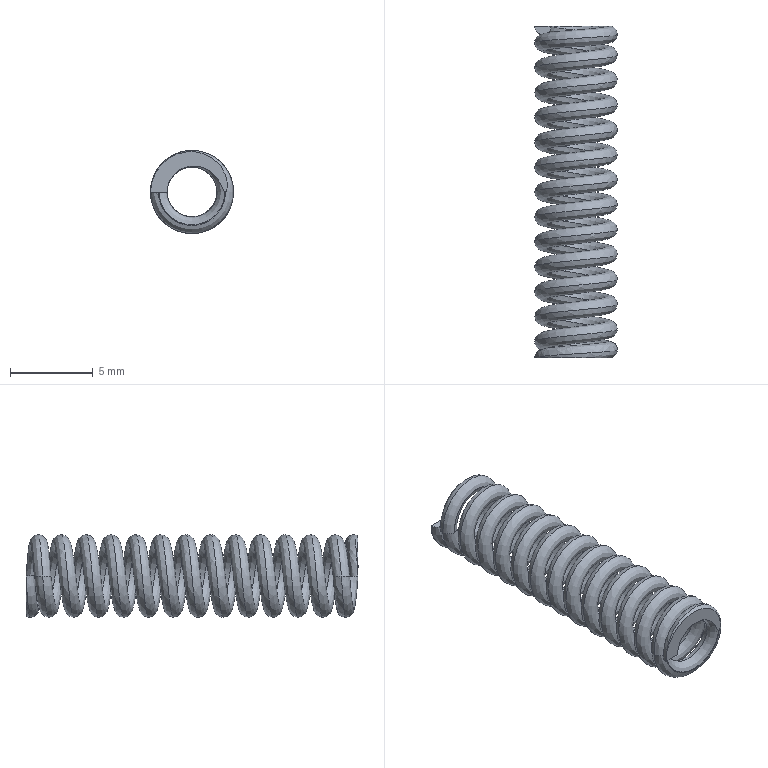Part | SolidWorks | features Sweep 3, ICE 1 | 1 solid | 18 faces | volume 136.283 mm3 | spline 14 | plane 4